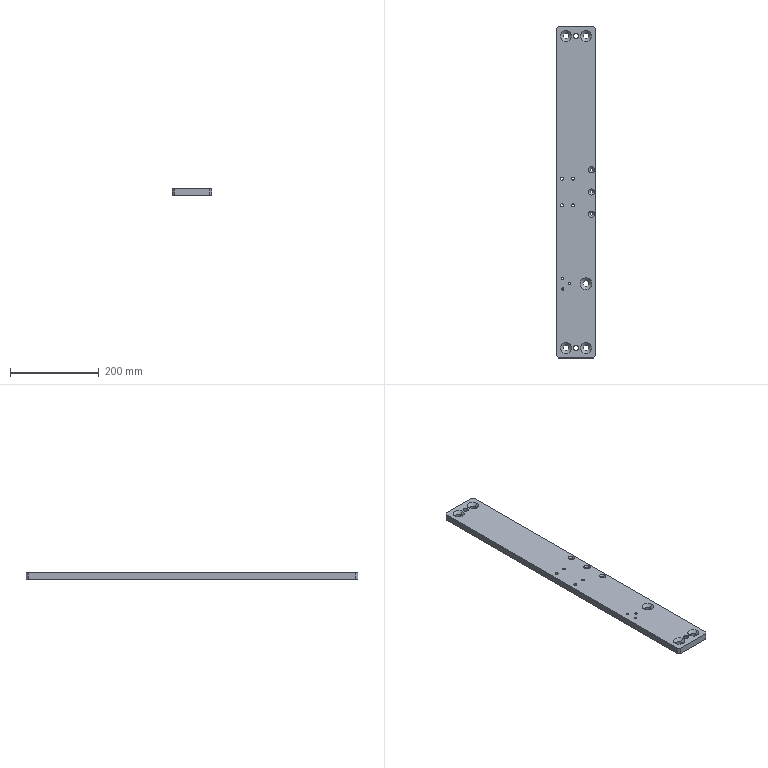Part | STEP file | 1 solid | 64 faces | box 90 x 748 x 15 mm | volume 986342 mm3 | cylinder 34 | cone 20 | plane 10 | commonest cylinder face diameters 6.8 x8 13 x8 5 x6 6.6 x6 10.2 x4 13.5 x2